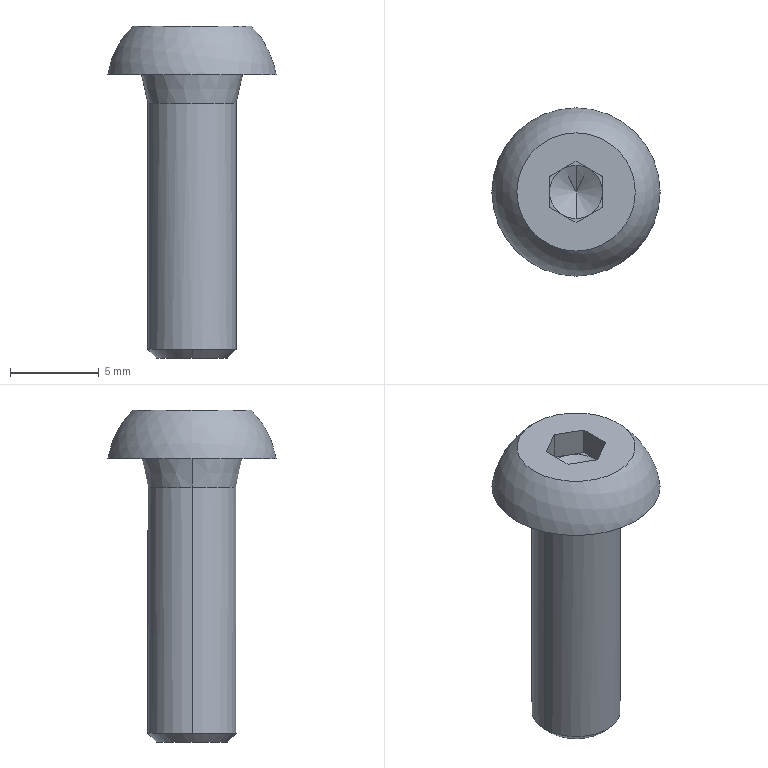Part | SolidWorks | features BaseBody 1 | 1 solid | 24 faces | box 9.5 x 9.5 x 18.75 mm | volume 459.314 mm3 | plane 15 | cone 6 | cylinder 2 | sphere 1 | commonest cylinder face diameters 5 x2
STEP:
#1=CARTESIAN_POINT('',(0.,2.5,-13.91));
#2=VERTEX_POINT('',#1);
#3=CARTESIAN_POINT('',(-2.5,0.,-13.91));
#4=VERTEX_POINT('',#3);
#5=CARTESIAN_POINT('',(0.,0.,-13.91));
#6=DIRECTION('',(0.,0.,1.));
#7=DIRECTION('',(1.,0.,0.));
#8=AXIS2_PLACEMENT_3D('',#5,#6,#7);
#9=CIRCLE('',#8,2.5);
#10=EDGE_CURVE('',#2,#4,#9,.T.);
#11=ORIENTED_EDGE('',*,*,#10,.T.);
#12=CARTESIAN_POINT('',(-2.5,0.,0.));
#13=VERTEX_POINT('',#12);
#14=CARTESIAN_POINT('',(-2.5,0.,-14.4));
#15=DIRECTION('',(0.,0.,1.));
#16=VECTOR('',#15,1000.);
#17=LINE('',#14,#16);
#18=EDGE_CURVE('',#4,#13,#17,.T.);
#19=ORIENTED_EDGE('',*,*,#18,.T.);
#20=CARTESIAN_POINT('',(2.5,0.,0.));
#21=VERTEX_POINT('',#20);
#22=CARTESIAN_POINT('',(0.,0.,0.));
#23=DIRECTION('',(0.,0.,-1.));
#24=DIRECTION('',(1.,0.,0.));
#25=AXIS2_PLACEMENT_3D('',#22,#23,#24);
#26=CIRCLE('',#25,2.5);
#27=EDGE_CURVE('',#13,#21,#26,.T.);
#28=ORIENTED_EDGE('',*,*,#27,.T.);
#29=CARTESIAN_POINT('',(2.5,0.,-13.91));
#30=VERTEX_POINT('',#29);
#31=CARTESIAN_POINT('',(2.5,0.,-14.4));
#32=DIRECTION('',(0.,0.,1.));
#33=VECTOR('',#32,1000.);
#34=LINE('',#31,#33);
#35=EDGE_CURVE('',#30,#21,#34,.T.);
#36=ORIENTED_EDGE('',*,*,#35,.F.);
#37=CARTESIAN_POINT('',(0.,0.,-13.91));
#38=DIRECTION('',(0.,0.,1.));
#39=DIRECTION('',(1.,0.,0.));
#40=AXIS2_PLACEMENT_3D('',#37,#38,#39);
#41=CIRCLE('',#40,2.5);
#42=EDGE_CURVE('',#30,#2,#41,.T.);
#43=ORIENTED_EDGE('',*,*,#42,.T.);
#44=EDGE_LOOP('',(#11,#19,#28,#36,#43));
#45=FACE_OUTER_BOUND('',#44,.T.);
#46=CARTESIAN_POINT('',(0.,0.,-14.4));
#47=DIRECTION('',(0.,0.,1.));
#48=DIRECTION('',(1.,0.,0.));
#49=AXIS2_PLACEMENT_3D('',#46,#47,#48);
#50=CYLINDRICAL_SURFACE('',#49,2.5);
#51=ADVANCED_FACE('',(#45),#50,.T.);
#52=ORIENTED_EDGE('',*,*,#27,.F.);
#53=CARTESIAN_POINT('',(-2.85,0.,1.6));
#54=VERTEX_POINT('',#53);
#55=CARTESIAN_POINT('',(-2.85,0.,1.6));
#56=DIRECTION('',(-0.2137,0.,0.9769));
#57=VECTOR('',#56,1000.);
#58=LINE('',#55,#57);
#59=EDGE_CURVE('',#13,#54,#58,.T.);
#60=ORIENTED_EDGE('',*,*,#59,.T.);
#61=CARTESIAN_POINT('',(2.85,0.,1.6));
#62=VERTEX_POINT('',#61);
#63=CARTESIAN_POINT('',(0.,0.,1.6));
#64=DIRECTION('',(0.,0.,-1.));
#65=DIRECTION('',(1.,0.,0.));
#66=AXIS2_PLACEMENT_3D('',#63,#64,#65);
#67=CIRCLE('',#66,2.85);
#68=EDGE_CURVE('',#54,#62,#67,.T.);
#69=ORIENTED_EDGE('',*,*,#68,.T.);
#70=CARTESIAN_POINT('',(2.85,0.,1.6));
#71=DIRECTION('',(0.2137,0.,0.9769));
#72=VECTOR('',#71,1000.);
#73=LINE('',#70,#72);
#74=EDGE_CURVE('',#21,#62,#73,.T.);
#75=ORIENTED_EDGE('',*,*,#74,.F.);
#76=EDGE_LOOP('',(#52,#60,#69,#75));
#77=FACE_OUTER_BOUND('',#76,.T.);
#78=CARTESIAN_POINT('',(0.,0.,1.6));
#79=DIRECTION('',(0.,0.,1.));
#80=DIRECTION('',(1.,0.,0.));
#81=AXIS2_PLACEMENT_3D('',#78,#79,#80);
#82=CONICAL_SURFACE('',#81,2.85,0.2154);
#83=ADVANCED_FACE('',(#77),#82,.T.);
#84=CARTESIAN_POINT('',(0.,-2.009,-14.4));
#85=VERTEX_POINT('',#84);
#86=CARTESIAN_POINT('',(0.,2.009,-14.4));
#87=VERTEX_POINT('',#86);
#88=CARTESIAN_POINT('',(0.,0.,-14.4));
#89=DIRECTION('',(0.,0.,1.));
#90=DIRECTION('',(0.,-1.,0.));
#91=AXIS2_PLACEMENT_3D('',#88,#89,#90);
#92=CIRCLE('',#91,2.009);
#93=EDGE_CURVE('',#85,#87,#92,.T.);
#94=ORIENTED_EDGE('',*,*,#93,.T.);
#95=CARTESIAN_POINT('',(0.,2.5,-13.909));
#96=DIRECTION('',(0.,0.7071,0.7071));
#97=VECTOR('',#96,1000.);
#98=LINE('',#95,#97);
#99=EDGE_CURVE('',#87,#2,#98,.T.);
#100=ORIENTED_EDGE('',*,*,#99,.T.);
#101=ORIENTED_EDGE('',*,*,#42,.F.);
#102=CARTESIAN_POINT('',(0.,-2.5,-13.91));
#103=VERTEX_POINT('',#102);
#104=CARTESIAN_POINT('',(0.,0.,-13.91));
#105=DIRECTION('',(0.,0.,1.));
#106=DIRECTION('',(1.,0.,0.));
#107=AXIS2_PLACEMENT_3D('',#104,#105,#106);
#108=CIRCLE('',#107,2.5);
#109=EDGE_CURVE('',#103,#30,#108,.T.);
#110=ORIENTED_EDGE('',*,*,#109,.F.);
#111=CARTESIAN_POINT('',(0.,-2.5,-13.909));
#112=DIRECTION('',(0.,-0.7071,0.7071));
#113=VECTOR('',#112,1000.);
#114=LINE('',#111,#113);
#115=EDGE_CURVE('',#85,#103,#114,.T.);
#116=ORIENTED_EDGE('',*,*,#115,.F.);
#117=EDGE_LOOP('',(#94,#100,#101,#110,#116));
#118=FACE_OUTER_BOUND('',#117,.T.);
#119=CARTESIAN_POINT('',(0.,0.,-13.909));
#120=DIRECTION('',(0.,0.,1.));
#121=DIRECTION('',(0.,-1.,0.));
#122=AXIS2_PLACEMENT_3D('',#119,#120,#121);
#123=CONICAL_SURFACE('',#122,2.5,0.7854);
#124=ADVANCED_FACE('',(#118),#123,.T.);
#125=CARTESIAN_POINT('',(0.,0.,1.924));
#126=VERTEX_POINT('',#125);
#127=CARTESIAN_POINT('',(0.,-1.5,2.79));
#128=VERTEX_POINT('',#127);
#129=CARTESIAN_POINT('',(0.,-1.5,2.79));
#130=DIRECTION('',(0.,-0.866,0.5));
#131=VECTOR('',#130,1000.);
#132=LINE('',#129,#131);
#133=EDGE_CURVE('',#126,#128,#132,.T.);
#134=ORIENTED_EDGE('',*,*,#133,.F.);
#135=CARTESIAN_POINT('',(0.,1.5,2.79));
#136=VERTEX_POINT('',#135);
#137=CARTESIAN_POINT('',(0.,1.5,2.79));
#138=DIRECTION('',(0.,0.866,0.5));
#139=VECTOR('',#138,1000.);
#140=LINE('',#137,#139);
#141=EDGE_CURVE('',#126,#136,#140,.T.);
#142=ORIENTED_EDGE('',*,*,#141,.T.);
#143=CARTESIAN_POINT('',(-0.75,1.299,2.79));
#144=VERTEX_POINT('',#143);
#145=CARTESIAN_POINT('',(0.,0.,2.79));
#146=DIRECTION('',(0.,0.,-1.));
#147=DIRECTION('',(0.,-1.,0.));
#148=AXIS2_PLACEMENT_3D('',#145,#146,#147);
#149=CIRCLE('',#148,1.5);
#150=EDGE_CURVE('',#144,#136,#149,.T.);
#151=ORIENTED_EDGE('',*,*,#150,.F.);
#152=CARTESIAN_POINT('',(-1.5,0.,2.79));
#153=VERTEX_POINT('',#152);
#154=CARTESIAN_POINT('',(0.,0.,2.79));
#155=DIRECTION('',(0.,0.,-1.));
#156=DIRECTION('',(0.,-1.,0.));
#157=AXIS2_PLACEMENT_3D('',#154,#155,#156);
#158=CIRCLE('',#157,1.5);
#159=EDGE_CURVE('',#153,#144,#158,.T.);
#160=ORIENTED_EDGE('',*,*,#159,.F.);
#161=CARTESIAN_POINT('',(-0.75,-1.299,2.79));
#162=VERTEX_POINT('',#161);
#163=CARTESIAN_POINT('',(0.,0.,2.79));
#164=DIRECTION('',(0.,0.,-1.));
#165=DIRECTION('',(0.,-1.,0.));
#166=AXIS2_PLACEMENT_3D('',#163,#164,#165);
#167=CIRCLE('',#166,1.5);
#168=EDGE_CURVE('',#162,#153,#167,.T.);
#169=ORIENTED_EDGE('',*,*,#168,.F.);
#170=CARTESIAN_POINT('',(0.,0.,2.79));
#171=DIRECTION('',(0.,0.,-1.));
#172=DIRECTION('',(0.,-1.,0.));
#173=AXIS2_PLACEMENT_3D('',#170,#171,#172);
#174=CIRCLE('',#173,1.5);
#175=EDGE_CURVE('',#128,#162,#174,.T.);
#176=ORIENTED_EDGE('',*,*,#175,.F.);
#177=EDGE_LOOP('',(#134,#142,#151,#160,#169,#176));
#178=FACE_OUTER_BOUND('',#177,.T.);
#179=CARTESIAN_POINT('',(0.,0.,2.79));
#180=DIRECTION('',(0.,0.,1.));
#181=DIRECTION('',(0.,-1.,0.));
#182=AXIS2_PLACEMENT_3D('',#179,#180,#181);
#183=CONICAL_SURFACE('',#182,1.5,1.047);
#184=ADVANCED_FACE('',(#178),#183,.F.);
#185=ORIENTED_EDGE('',*,*,#18,.F.);
#186=CARTESIAN_POINT('',(0.,0.,-13.91));
#187=DIRECTION('',(0.,0.,1.));
#188=DIRECTION('',(1.,0.,0.));
#189=AXIS2_PLACEMENT_3D('',#186,#187,#188);
#190=CIRCLE('',#189,2.5);
#191=EDGE_CURVE('',#4,#103,#190,.T.);
#192=ORIENTED_EDGE('',*,*,#191,.T.);
#193=ORIENTED_EDGE('',*,*,#109,.T.);
#194=ORIENTED_EDGE('',*,*,#35,.T.);
#195=CARTESIAN_POINT('',(0.,0.,0.));
#196=DIRECTION('',(0.,0.,-1.));
#197=DIRECTION('',(1.,0.,0.));
#198=AXIS2_PLACEMENT_3D('',#195,#196,#197);
#199=CIRCLE('',#198,2.5);
#200=EDGE_CURVE('',#21,#13,#199,.T.);
#201=ORIENTED_EDGE('',*,*,#200,.T.);
#202=EDGE_LOOP('',(#185,#192,#193,#194,#201));
#203=FACE_OUTER_BOUND('',#202,.T.);
#204=CARTESIAN_POINT('',(0.,0.,-14.4));
#205=DIRECTION('',(0.,0.,1.));
#206=DIRECTION('',(1.,0.,0.));
#207=AXIS2_PLACEMENT_3D('',#204,#205,#206);
#208=CYLINDRICAL_SURFACE('',#207,2.5);
#209=ADVANCED_FACE('',(#203),#208,.T.);
#210=ORIENTED_EDGE('',*,*,#59,.F.);
#211=ORIENTED_EDGE('',*,*,#200,.F.);
#212=ORIENTED_EDGE('',*,*,#74,.T.);
#213=CARTESIAN_POINT('',(0.,0.,1.6));
#214=DIRECTION('',(0.,0.,-1.));
#215=DIRECTION('',(1.,0.,0.));
#216=AXIS2_PLACEMENT_3D('',#213,#214,#215);
#217=CIRCLE('',#216,2.85);
#218=EDGE_CURVE('',#62,#54,#217,.T.);
#219=ORIENTED_EDGE('',*,*,#218,.T.);
#220=EDGE_LOOP('',(#210,#211,#212,#219));
#221=FACE_OUTER_BOUND('',#220,.T.);
#222=CARTESIAN_POINT('',(0.,0.,1.6));
#223=DIRECTION('',(0.,0.,1.));
#224=DIRECTION('',(1.,0.,0.));
#225=AXIS2_PLACEMENT_3D('',#222,#223,#224);
#226=CONICAL_SURFACE('',#225,2.85,0.2154);
#227=ADVANCED_FACE('',(#221),#226,.T.);
#228=ORIENTED_EDGE('',*,*,#99,.F.);
#229=CARTESIAN_POINT('',(0.,0.,-14.4));
#230=DIRECTION('',(0.,0.,1.));
#231=DIRECTION('',(0.,-1.,0.));
#232=AXIS2_PLACEMENT_3D('',#229,#230,#231);
#233=CIRCLE('',#232,2.009);
#234=EDGE_CURVE('',#87,#85,#233,.T.);
#235=ORIENTED_EDGE('',*,*,#234,.T.);
#236=ORIENTED_EDGE('',*,*,#115,.T.);
#237=ORIENTED_EDGE('',*,*,#191,.F.);
#238=ORIENTED_EDGE('',*,*,#10,.F.);
#239=EDGE_LOOP('',(#228,#235,#236,#237,#238));
#240=FACE_OUTER_BOUND('',#239,.T.);
#241=CARTESIAN_POINT('',(0.,0.,-13.909));
#242=DIRECTION('',(0.,0.,1.));
#243=DIRECTION('',(0.,-1.,0.));
#244=AXIS2_PLACEMENT_3D('',#241,#242,#243);
#245=CONICAL_SURFACE('',#244,2.5,0.7854);
#246=ADVANCED_FACE('',(#240),#245,.T.);
#247=CARTESIAN_POINT('',(4.75,0.,1.6));
#248=VERTEX_POINT('',#247);
#249=CARTESIAN_POINT('',(-4.75,0.,1.6));
#250=VERTEX_POINT('',#249);
#251=CARTESIAN_POINT('',(0.,0.,1.6));
#252=DIRECTION('',(0.,0.,1.));
#253=DIRECTION('',(1.,0.,0.));
#254=AXIS2_PLACEMENT_3D('',#251,#252,#253);
#255=CIRCLE('',#254,4.75);
#256=EDGE_CURVE('',#248,#250,#255,.T.);
#257=ORIENTED_EDGE('',*,*,#256,.F.);
#258=CARTESIAN_POINT('',(0.,0.,1.6));
#259=DIRECTION('',(0.,0.,1.));
#260=DIRECTION('',(1.,0.,0.));
#261=AXIS2_PLACEMENT_3D('',#258,#259,#260);
#262=CIRCLE('',#261,4.75);
#263=EDGE_CURVE('',#250,#248,#262,.T.);
#264=ORIENTED_EDGE('',*,*,#263,.F.);
#265=EDGE_LOOP('',(#257,#264));
#266=FACE_OUTER_BOUND('',#265,.T.);
#267=ORIENTED_EDGE('',*,*,#218,.F.);
#268=ORIENTED_EDGE('',*,*,#68,.F.);
#269=EDGE_LOOP('',(#267,#268));
#270=FACE_BOUND('',#269,.T.);
#271=CARTESIAN_POINT('',(0.,4.75,1.6));
#272=DIRECTION('',(0.,0.,1.));
#273=DIRECTION('',(1.,0.,0.));
#274=AXIS2_PLACEMENT_3D('',#271,#272,#273);
#275=PLANE('',#274);
#276=ADVANCED_FACE('',(#266,#270),#275,.F.);
#277=ORIENTED_EDGE('',*,*,#93,.F.);
#278=ORIENTED_EDGE('',*,*,#234,.F.);
#279=EDGE_LOOP('',(#277,#278));
#280=FACE_OUTER_BOUND('',#279,.T.);
#281=CARTESIAN_POINT('',(2.5,0.,-14.4));
#282=DIRECTION('',(0.,0.,-1.));
#283=DIRECTION('',(-1.,0.,0.));
#284=AXIS2_PLACEMENT_3D('',#281,#282,#283);
#285=PLANE('',#284);
#286=ADVANCED_FACE('',(#280),#285,.T.);
#287=CARTESIAN_POINT('',(-3.339,0.,4.35));
#288=VERTEX_POINT('',#287);
#289=CARTESIAN_POINT('',(3.339,0.,4.35));
#290=VERTEX_POINT('',#289);
#291=CARTESIAN_POINT('',(0.,0.,4.35));
#292=DIRECTION('',(0.,0.,-1.));
#293=DIRECTION('',(-1.,0.,0.));
#294=AXIS2_PLACEMENT_3D('',#291,#292,#293);
#295=CIRCLE('',#294,3.339);
#296=EDGE_CURVE('',#288,#290,#295,.T.);
#297=ORIENTED_EDGE('',*,*,#296,.T.);
#298=CARTESIAN_POINT('',(0.,0.,4.35));
#299=DIRECTION('',(0.,0.,-1.));
#300=DIRECTION('',(-1.,0.,0.));
#301=AXIS2_PLACEMENT_3D('',#298,#299,#300);
#302=CIRCLE('',#301,3.339);
#303=EDGE_CURVE('',#290,#288,#302,.T.);
#304=ORIENTED_EDGE('',*,*,#303,.T.);
#305=EDGE_LOOP('',(#297,#304));
#306=FACE_BOUND('',#305,.T.);
#307=ORIENTED_EDGE('',*,*,#256,.T.);
#308=ORIENTED_EDGE('',*,*,#263,.T.);
#309=EDGE_LOOP('',(#307,#308));
#310=FACE_OUTER_BOUND('',#309,.T.);
#311=CARTESIAN_POINT('',(0.,0.,0.9));
#312=DIRECTION('',(0.1289,0.,0.9917));
#313=DIRECTION('',(-0.9917,0.,0.1289));
#314=AXIS2_PLACEMENT_3D('',#311,#312,#313);
#315=SPHERICAL_SURFACE('',#314,4.801);
#316=ADVANCED_FACE('',(#306,#310),#315,.T.);
#317=ORIENTED_EDGE('',*,*,#296,.F.);
#318=ORIENTED_EDGE('',*,*,#303,.F.);
#319=EDGE_LOOP('',(#317,#318));
#320=FACE_OUTER_BOUND('',#319,.T.);
#321=CARTESIAN_POINT('',(0.,-1.732,4.35));
#322=VERTEX_POINT('',#321);
#323=CARTESIAN_POINT('',(1.5,-0.866,4.35));
#324=VERTEX_POINT('',#323);
#325=CARTESIAN_POINT('',(0.,-1.732,4.35));
#326=DIRECTION('',(0.866,0.5,0.));
#327=VECTOR('',#326,1000.);
#328=LINE('',#325,#327);
#329=EDGE_CURVE('',#322,#324,#328,.T.);
#330=ORIENTED_EDGE('',*,*,#329,.F.);
#331=CARTESIAN_POINT('',(-1.5,-0.866,4.35));
#332=VERTEX_POINT('',#331);
#333=CARTESIAN_POINT('',(-1.5,-0.866,4.35));
#334=DIRECTION('',(0.866,-0.5,0.));
#335=VECTOR('',#334,1000.);
#336=LINE('',#333,#335);
#337=EDGE_CURVE('',#332,#322,#336,.T.);
#338=ORIENTED_EDGE('',*,*,#337,.F.);
#339=CARTESIAN_POINT('',(-1.5,0.866,4.35));
#340=VERTEX_POINT('',#339);
#341=CARTESIAN_POINT('',(-1.5,0.,4.35));
#342=DIRECTION('',(0.,-1.,0.));
#343=VECTOR('',#342,1000.);
#344=LINE('',#341,#343);
#345=EDGE_CURVE('',#340,#332,#344,.T.);
#346=ORIENTED_EDGE('',*,*,#345,.F.);
#347=CARTESIAN_POINT('',(0.,1.732,4.35));
#348=VERTEX_POINT('',#347);
#349=CARTESIAN_POINT('',(0.,1.732,4.35));
#350=DIRECTION('',(-0.866,-0.5,0.));
#351=VECTOR('',#350,1000.);
#352=LINE('',#349,#351);
#353=EDGE_CURVE('',#348,#340,#352,.T.);
#354=ORIENTED_EDGE('',*,*,#353,.F.);
#355=CARTESIAN_POINT('',(1.5,0.866,4.35));
#356=VERTEX_POINT('',#355);
#357=CARTESIAN_POINT('',(1.5,0.866,4.35));
#358=DIRECTION('',(-0.866,0.5,0.));
#359=VECTOR('',#358,1000.);
#360=LINE('',#357,#359);
#361=EDGE_CURVE('',#356,#348,#360,.T.);
#362=ORIENTED_EDGE('',*,*,#361,.F.);
#363=CARTESIAN_POINT('',(1.5,0.,4.35));
#364=DIRECTION('',(0.,1.,0.));
#365=VECTOR('',#364,1000.);
#366=LINE('',#363,#365);
#367=EDGE_CURVE('',#324,#356,#366,.T.);
#368=ORIENTED_EDGE('',*,*,#367,.F.);
#369=EDGE_LOOP('',(#330,#338,#346,#354,#362,#368));
#370=FACE_BOUND('',#369,.T.);
#371=CARTESIAN_POINT('',(0.,0.,4.35));
#372=DIRECTION('',(0.,0.,-1.));
#373=DIRECTION('',(-1.,0.,0.));
#374=AXIS2_PLACEMENT_3D('',#371,#372,#373);
#375=PLANE('',#374);
#376=ADVANCED_FACE('',(#320,#370),#375,.F.);
#377=CARTESIAN_POINT('',(1.5,0.866,2.79));
#378=VERTEX_POINT('',#377);
#379=CARTESIAN_POINT('',(1.5,0.866,2.79));
#380=DIRECTION('',(0.,0.,1.));
#381=VECTOR('',#380,1000.);
#382=LINE('',#379,#381);
#383=EDGE_CURVE('',#378,#356,#382,.T.);
#384=ORIENTED_EDGE('',*,*,#383,.F.);
#385=CARTESIAN_POINT('',(1.5,0.,2.79));
#386=VERTEX_POINT('',#385);
#387=CARTESIAN_POINT('',(1.5,-0.866,2.79));
#388=DIRECTION('',(0.,1.,0.));
#389=VECTOR('',#388,1000.);
#390=LINE('',#387,#389);
#391=EDGE_CURVE('',#386,#378,#390,.T.);
#392=ORIENTED_EDGE('',*,*,#391,.F.);
#393=CARTESIAN_POINT('',(1.5,-0.866,2.79));
#394=VERTEX_POINT('',#393);
#395=CARTESIAN_POINT('',(1.5,-0.866,2.79));
#396=DIRECTION('',(0.,1.,0.));
#397=VECTOR('',#396,1000.);
#398=LINE('',#395,#397);
#399=EDGE_CURVE('',#394,#386,#398,.T.);
#400=ORIENTED_EDGE('',*,*,#399,.F.);
#401=CARTESIAN_POINT('',(1.5,-0.866,2.79));
#402=DIRECTION('',(0.,0.,-1.));
#403=VECTOR('',#402,1000.);
#404=LINE('',#401,#403);
#405=EDGE_CURVE('',#324,#394,#404,.T.);
#406=ORIENTED_EDGE('',*,*,#405,.F.);
#407=ORIENTED_EDGE('',*,*,#367,.T.);
#408=EDGE_LOOP('',(#384,#392,#400,#406,#407));
#409=FACE_OUTER_BOUND('',#408,.T.);
#410=CARTESIAN_POINT('',(1.5,-0.866,2.79));
#411=DIRECTION('',(1.,0.,0.));
#412=DIRECTION('',(0.,0.,-1.));
#413=AXIS2_PLACEMENT_3D('',#410,#411,#412);
#414=PLANE('',#413);
#415=ADVANCED_FACE('',(#409),#414,.F.);
#416=ORIENTED_EDGE('',*,*,#405,.T.);
#417=CARTESIAN_POINT('',(0.75,-1.299,2.79));
#418=VERTEX_POINT('',#417);
#419=CARTESIAN_POINT('',(0.,-1.732,2.79));
#420=DIRECTION('',(0.866,0.5,0.));
#421=VECTOR('',#420,1000.);
#422=LINE('',#419,#421);
#423=EDGE_CURVE('',#418,#394,#422,.T.);
#424=ORIENTED_EDGE('',*,*,#423,.F.);
#425=CARTESIAN_POINT('',(0.,-1.732,2.79));
#426=VERTEX_POINT('',#425);
#427=CARTESIAN_POINT('',(0.,-1.732,2.79));
#428=DIRECTION('',(0.866,0.5,0.));
#429=VECTOR('',#428,1000.);
#430=LINE('',#427,#429);
#431=EDGE_CURVE('',#426,#418,#430,.T.);
#432=ORIENTED_EDGE('',*,*,#431,.F.);
#433=CARTESIAN_POINT('',(0.,-1.732,2.79));
#434=DIRECTION('',(0.,0.,-1.));
#435=VECTOR('',#434,1000.);
#436=LINE('',#433,#435);
#437=EDGE_CURVE('',#322,#426,#436,.T.);
#438=ORIENTED_EDGE('',*,*,#437,.F.);
#439=ORIENTED_EDGE('',*,*,#329,.T.);
#440=EDGE_LOOP('',(#416,#424,#432,#438,#439));
#441=FACE_OUTER_BOUND('',#440,.T.);
#442=CARTESIAN_POINT('',(0.,-1.732,2.79));
#443=DIRECTION('',(0.5,-0.866,0.));
#444=DIRECTION('',(0.866,0.5,0.));
#445=AXIS2_PLACEMENT_3D('',#442,#443,#444);
#446=PLANE('',#445);
#447=ADVANCED_FACE('',(#441),#446,.F.);
#448=ORIENTED_EDGE('',*,*,#437,.T.);
#449=CARTESIAN_POINT('',(-1.5,-0.866,2.79));
#450=DIRECTION('',(0.866,-0.5,0.));
#451=VECTOR('',#450,1000.);
#452=LINE('',#449,#451);
#453=EDGE_CURVE('',#162,#426,#452,.T.);
#454=ORIENTED_EDGE('',*,*,#453,.F.);
#455=CARTESIAN_POINT('',(-1.5,-0.866,2.79));
#456=VERTEX_POINT('',#455);
#457=CARTESIAN_POINT('',(-1.5,-0.866,2.79));
#458=DIRECTION('',(0.866,-0.5,0.));
#459=VECTOR('',#458,1000.);
#460=LINE('',#457,#459);
#461=EDGE_CURVE('',#456,#162,#460,.T.);
#462=ORIENTED_EDGE('',*,*,#461,.F.);
#463=CARTESIAN_POINT('',(-1.5,-0.866,2.79));
#464=DIRECTION('',(0.,0.,-1.));
#465=VECTOR('',#464,1000.);
#466=LINE('',#463,#465);
#467=EDGE_CURVE('',#332,#456,#466,.T.);
#468=ORIENTED_EDGE('',*,*,#467,.F.);
#469=ORIENTED_EDGE('',*,*,#337,.T.);
#470=EDGE_LOOP('',(#448,#454,#462,#468,#469));
#471=FACE_OUTER_BOUND('',#470,.T.);
#472=CARTESIAN_POINT('',(-1.5,-0.866,2.79));
#473=DIRECTION('',(-0.5,-0.866,0.));
#474=DIRECTION('',(0.866,-0.5,0.));
#475=AXIS2_PLACEMENT_3D('',#472,#473,#474);
#476=PLANE('',#475);
#477=ADVANCED_FACE('',(#471),#476,.F.);
#478=ORIENTED_EDGE('',*,*,#467,.T.);
#479=CARTESIAN_POINT('',(-1.5,0.866,2.79));
#480=DIRECTION('',(0.,-1.,0.));
#481=VECTOR('',#480,1000.);
#482=LINE('',#479,#481);
#483=EDGE_CURVE('',#153,#456,#482,.T.);
#484=ORIENTED_EDGE('',*,*,#483,.F.);
#485=CARTESIAN_POINT('',(-1.5,0.866,2.79));
#486=VERTEX_POINT('',#485);
#487=CARTESIAN_POINT('',(-1.5,0.866,2.79));
#488=DIRECTION('',(0.,-1.,0.));
#489=VECTOR('',#488,1000.);
#490=LINE('',#487,#489);
#491=EDGE_CURVE('',#486,#153,#490,.T.);
#492=ORIENTED_EDGE('',*,*,#491,.F.);
#493=CARTESIAN_POINT('',(-1.5,0.866,2.79));
#494=DIRECTION('',(0.,0.,-1.));
#495=VECTOR('',#494,1000.);
#496=LINE('',#493,#495);
#497=EDGE_CURVE('',#340,#486,#496,.T.);
#498=ORIENTED_EDGE('',*,*,#497,.F.);
#499=ORIENTED_EDGE('',*,*,#345,.T.);
#500=EDGE_LOOP('',(#478,#484,#492,#498,#499));
#501=FACE_OUTER_BOUND('',#500,.T.);
#502=CARTESIAN_POINT('',(-1.5,0.866,2.79));
#503=DIRECTION('',(-1.,0.,0.));
#504=DIRECTION('',(0.,-1.,0.));
#505=AXIS2_PLACEMENT_3D('',#502,#503,#504);
#506=PLANE('',#505);
#507=ADVANCED_FACE('',(#501),#506,.F.);
#508=ORIENTED_EDGE('',*,*,#497,.T.);
#509=CARTESIAN_POINT('',(0.,1.732,2.79));
#510=DIRECTION('',(-0.866,-0.5,0.));
#511=VECTOR('',#510,1000.);
#512=LINE('',#509,#511);
#513=EDGE_CURVE('',#144,#486,#512,.T.);
#514=ORIENTED_EDGE('',*,*,#513,.F.);
#515=CARTESIAN_POINT('',(0.,1.732,2.79));
#516=VERTEX_POINT('',#515);
#517=CARTESIAN_POINT('',(0.,1.732,2.79));
#518=DIRECTION('',(-0.866,-0.5,0.));
#519=VECTOR('',#518,1000.);
#520=LINE('',#517,#519);
#521=EDGE_CURVE('',#516,#144,#520,.T.);
#522=ORIENTED_EDGE('',*,*,#521,.F.);
#523=CARTESIAN_POINT('',(0.,1.732,2.79));
#524=DIRECTION('',(0.,0.,-1.));
#525=VECTOR('',#524,1000.);
#526=LINE('',#523,#525);
#527=EDGE_CURVE('',#348,#516,#526,.T.);
#528=ORIENTED_EDGE('',*,*,#527,.F.);
#529=ORIENTED_EDGE('',*,*,#353,.T.);
#530=EDGE_LOOP('',(#508,#514,#522,#528,#529));
#531=FACE_OUTER_BOUND('',#530,.T.);
#532=CARTESIAN_POINT('',(0.,1.732,2.79));
#533=DIRECTION('',(-0.5,0.866,0.));
#534=DIRECTION('',(-0.866,-0.5,0.));
#535=AXIS2_PLACEMENT_3D('',#532,#533,#534);
#536=PLANE('',#535);
#537=ADVANCED_FACE('',(#531),#536,.F.);
#538=ORIENTED_EDGE('',*,*,#527,.T.);
#539=CARTESIAN_POINT('',(0.75,1.299,2.79));
#540=VERTEX_POINT('',#539);
#541=CARTESIAN_POINT('',(1.5,0.866,2.79));
#542=DIRECTION('',(-0.866,0.5,0.));
#543=VECTOR('',#542,1000.);
#544=LINE('',#541,#543);
#545=EDGE_CURVE('',#540,#516,#544,.T.);
#546=ORIENTED_EDGE('',*,*,#545,.F.);
#547=CARTESIAN_POINT('',(1.5,0.866,2.79));
#548=DIRECTION('',(-0.866,0.5,0.));
#549=VECTOR('',#548,1000.);
#550=LINE('',#547,#549);
#551=EDGE_CURVE('',#378,#540,#550,.T.);
#552=ORIENTED_EDGE('',*,*,#551,.F.);
#553=ORIENTED_EDGE('',*,*,#383,.T.);
#554=ORIENTED_EDGE('',*,*,#361,.T.);
#555=EDGE_LOOP('',(#538,#546,#552,#553,#554));
#556=FACE_OUTER_BOUND('',#555,.T.);
#557=CARTESIAN_POINT('',(1.5,0.866,2.79));
#558=DIRECTION('',(0.5,0.866,0.));
#559=DIRECTION('',(-0.866,0.5,0.));
#560=AXIS2_PLACEMENT_3D('',#557,#558,#559);
#561=PLANE('',#560);
#562=ADVANCED_FACE('',(#556),#561,.F.);
#563=CARTESIAN_POINT('',(0.,0.,2.79));
#564=DIRECTION('',(0.,0.,-1.));
#565=DIRECTION('',(0.,-1.,0.));
#566=AXIS2_PLACEMENT_3D('',#563,#564,#565);
#567=CIRCLE('',#566,1.5);
#568=EDGE_CURVE('',#540,#386,#567,.T.);
#569=ORIENTED_EDGE('',*,*,#568,.T.);
#570=ORIENTED_EDGE('',*,*,#391,.T.);
#571=ORIENTED_EDGE('',*,*,#551,.T.);
#572=EDGE_LOOP('',(#569,#570,#571));
#573=FACE_OUTER_BOUND('',#572,.T.);
#574=CARTESIAN_POINT('',(0.,0.,2.79));
#575=DIRECTION('',(0.,0.,1.));
#576=DIRECTION('',(1.,0.,0.));
#577=AXIS2_PLACEMENT_3D('',#574,#575,#576);
#578=PLANE('',#577);
#579=ADVANCED_FACE('',(#573),#578,.T.);
#580=CARTESIAN_POINT('',(0.,0.,2.79));
#581=DIRECTION('',(0.,0.,-1.));
#582=DIRECTION('',(0.,-1.,0.));
#583=AXIS2_PLACEMENT_3D('',#580,#581,#582);
#584=CIRCLE('',#583,1.5);
#585=EDGE_CURVE('',#386,#418,#584,.T.);
#586=ORIENTED_EDGE('',*,*,#585,.T.);
#587=ORIENTED_EDGE('',*,*,#423,.T.);
#588=ORIENTED_EDGE('',*,*,#399,.T.);
#589=EDGE_LOOP('',(#586,#587,#588));
#590=FACE_OUTER_BOUND('',#589,.T.);
#591=CARTESIAN_POINT('',(0.,0.,2.79));
#592=DIRECTION('',(0.,0.,1.));
#593=DIRECTION('',(1.,0.,0.));
#594=AXIS2_PLACEMENT_3D('',#591,#592,#593);
#595=PLANE('',#594);
#596=ADVANCED_FACE('',(#590),#595,.T.);
#597=CARTESIAN_POINT('',(0.,0.,2.79));
#598=DIRECTION('',(0.,0.,-1.));
#599=DIRECTION('',(0.,-1.,0.));
#600=AXIS2_PLACEMENT_3D('',#597,#598,#599);
#601=CIRCLE('',#600,1.5);
#602=EDGE_CURVE('',#418,#128,#601,.T.);
#603=ORIENTED_EDGE('',*,*,#602,.T.);
#604=ORIENTED_EDGE('',*,*,#175,.T.);
#605=ORIENTED_EDGE('',*,*,#453,.T.);
#606=ORIENTED_EDGE('',*,*,#431,.T.);
#607=EDGE_LOOP('',(#603,#604,#605,#606));
#608=FACE_OUTER_BOUND('',#607,.T.);
#609=CARTESIAN_POINT('',(0.,0.,2.79));
#610=DIRECTION('',(0.,0.,1.));
#611=DIRECTION('',(1.,0.,0.));
#612=AXIS2_PLACEMENT_3D('',#609,#610,#611);
#613=PLANE('',#612);
#614=ADVANCED_FACE('',(#608),#613,.T.);
#615=ORIENTED_EDGE('',*,*,#168,.T.);
#616=ORIENTED_EDGE('',*,*,#483,.T.);
#617=ORIENTED_EDGE('',*,*,#461,.T.);
#618=EDGE_LOOP('',(#615,#616,#617));
#619=FACE_OUTER_BOUND('',#618,.T.);
#620=CARTESIAN_POINT('',(0.,0.,2.79));
#621=DIRECTION('',(0.,0.,1.));
#622=DIRECTION('',(1.,0.,0.));
#623=AXIS2_PLACEMENT_3D('',#620,#621,#622);
#624=PLANE('',#623);
#625=ADVANCED_FACE('',(#619),#624,.T.);
#626=ORIENTED_EDGE('',*,*,#159,.T.);
#627=ORIENTED_EDGE('',*,*,#513,.T.);
#628=ORIENTED_EDGE('',*,*,#491,.T.);
#629=EDGE_LOOP('',(#626,#627,#628));
#630=FACE_OUTER_BOUND('',#629,.T.);
#631=CARTESIAN_POINT('',(0.,0.,2.79));
#632=DIRECTION('',(0.,0.,1.));
#633=DIRECTION('',(1.,0.,0.));
#634=AXIS2_PLACEMENT_3D('',#631,#632,#633);
#635=PLANE('',#634);
#636=ADVANCED_FACE('',(#630),#635,.T.);
#637=ORIENTED_EDGE('',*,*,#150,.T.);
#638=CARTESIAN_POINT('',(0.,0.,2.79));
#639=DIRECTION('',(0.,0.,-1.));
#640=DIRECTION('',(0.,-1.,0.));
#641=AXIS2_PLACEMENT_3D('',#638,#639,#640);
#642=CIRCLE('',#641,1.5);
#643=EDGE_CURVE('',#136,#540,#642,.T.);
#644=ORIENTED_EDGE('',*,*,#643,.T.);
#645=ORIENTED_EDGE('',*,*,#545,.T.);
#646=ORIENTED_EDGE('',*,*,#521,.T.);
#647=EDGE_LOOP('',(#637,#644,#645,#646));
#648=FACE_OUTER_BOUND('',#647,.T.);
#649=CARTESIAN_POINT('',(0.,0.,2.79));
#650=DIRECTION('',(0.,0.,1.));
#651=DIRECTION('',(1.,0.,0.));
#652=AXIS2_PLACEMENT_3D('',#649,#650,#651);
#653=PLANE('',#652);
#654=ADVANCED_FACE('',(#648),#653,.T.);
#655=ORIENTED_EDGE('',*,*,#141,.F.);
#656=ORIENTED_EDGE('',*,*,#133,.T.);
#657=ORIENTED_EDGE('',*,*,#602,.F.);
#658=ORIENTED_EDGE('',*,*,#585,.F.);
#659=ORIENTED_EDGE('',*,*,#568,.F.);
#660=ORIENTED_EDGE('',*,*,#643,.F.);
#661=EDGE_LOOP('',(#655,#656,#657,#658,#659,#660));
#662=FACE_OUTER_BOUND('',#661,.T.);
#663=CARTESIAN_POINT('',(0.,0.,2.79));
#664=DIRECTION('',(0.,0.,1.));
#665=DIRECTION('',(0.,-1.,0.));
#666=AXIS2_PLACEMENT_3D('',#663,#664,#665);
#667=CONICAL_SURFACE('',#666,1.5,1.047);
#668=ADVANCED_FACE('',(#662),#667,.F.);
#669=CLOSED_SHELL('',(#51,#83,#124,#184,#209,#227,#246,#276,#286,#316,#376,#415,#447,#477,#507,#537,#562,#579,#596,#614,#625,#636,#654,#668));
#670=MANIFOLD_SOLID_BREP('',#669);
#671=CARTESIAN_POINT('',(0.,0.,0.));
#672=DIRECTION('',(0.,0.,1.));
#673=DIRECTION('',(1.,0.,0.));
#674=AXIS2_PLACEMENT_3D('',#671,#672,#673);
#675=(LENGTH_UNIT()NAMED_UNIT(*)SI_UNIT(.MILLI.,.METRE.));
#676=UNCERTAINTY_MEASURE_WITH_UNIT(LENGTH_MEASURE(0.00001),#675,'','');
#677=(NAMED_UNIT(*)PLANE_ANGLE_UNIT()SI_UNIT($,.RADIAN.));
#678=(NAMED_UNIT(*)SI_UNIT($,.STERADIAN.)SOLID_ANGLE_UNIT());
#679=(GEOMETRIC_REPRESENTATION_CONTEXT(3)GLOBAL_UNCERTAINTY_ASSIGNED_CONTEXT((#676))GLOBAL_UNIT_ASSIGNED_CONTEXT((#675,#677,#678))REPRESENTATION_CONTEXT('',''));
#680=ADVANCED_BREP_SHAPE_REPRESENTATION('',(#670,#674),#679);